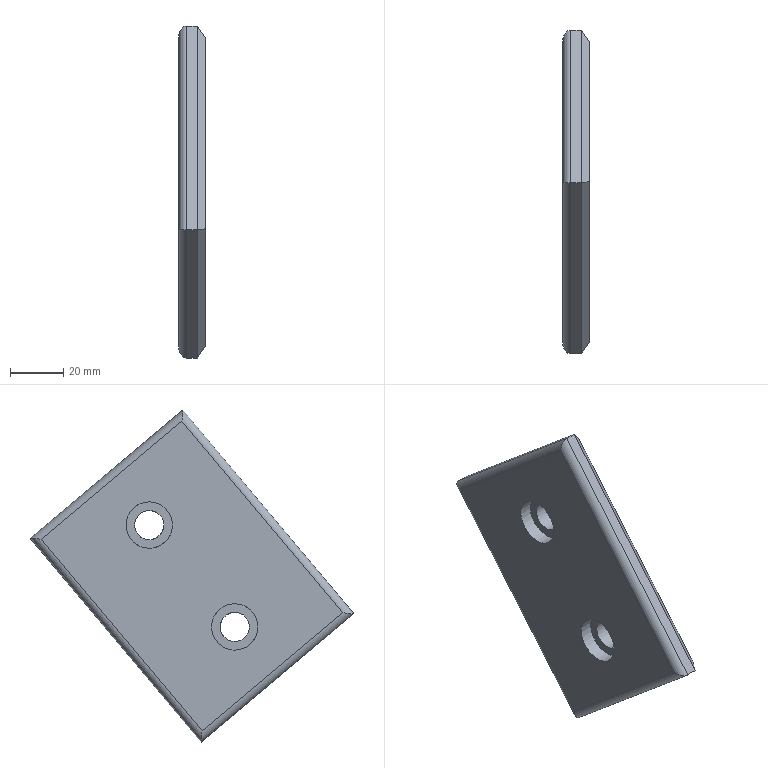Part | NX | features solid 2 | 1 solid | 20 faces | box 10 x 121.732 x 124.814 mm | volume 69440 mm3 | plane 12 | cylinder 8 | commonest cylinder face diameters 6 x4 11 x2 17.5 x2
STEP:
#1=CARTESIAN_POINT('',(-538.,288.281,-130.936));
#2=VERTEX_POINT('',#1);
#3=CARTESIAN_POINT('',(-542.,288.281,-130.936));
#4=VERTEX_POINT('',#3);
#5=CARTESIAN_POINT('',(-535.,288.281,-130.936));
#6=DIRECTION('',(-1.,0.,0.));
#7=VECTOR('',#6,1000.);
#8=LINE('',#5,#7);
#9=EDGE_CURVE('',#2,#4,#8,.T.);
#10=ORIENTED_EDGE('',*,*,#9,.T.);
#11=CARTESIAN_POINT('',(-542.,345.734,-179.146));
#12=VERTEX_POINT('',#11);
#13=CARTESIAN_POINT('',(-542.,288.281,-130.936));
#14=DIRECTION('',(0.,-0.766,0.6428));
#15=VECTOR('',#14,1000.);
#16=LINE('',#13,#15);
#17=EDGE_CURVE('',#12,#4,#16,.T.);
#18=ORIENTED_EDGE('',*,*,#17,.F.);
#19=CARTESIAN_POINT('',(-538.,345.734,-179.146));
#20=VERTEX_POINT('',#19);
#21=CARTESIAN_POINT('',(-535.,345.734,-179.146));
#22=DIRECTION('',(-1.,0.,0.));
#23=VECTOR('',#22,1000.);
#24=LINE('',#21,#23);
#25=EDGE_CURVE('',#20,#12,#24,.T.);
#26=ORIENTED_EDGE('',*,*,#25,.F.);
#27=CARTESIAN_POINT('',(-538.,345.734,-179.146));
#28=DIRECTION('',(0.,0.766,-0.6428));
#29=VECTOR('',#28,1000.);
#30=LINE('',#27,#29);
#31=EDGE_CURVE('',#2,#20,#30,.T.);
#32=ORIENTED_EDGE('',*,*,#31,.F.);
#33=EDGE_LOOP('',(#10,#18,#26,#32));
#34=FACE_BOUND('',#33,.T.);
#35=CARTESIAN_POINT('',(-535.,345.734,-179.146));
#36=DIRECTION('',(0.,0.6428,0.766));
#37=DIRECTION('',(0.,0.766,-0.6428));
#38=AXIS2_PLACEMENT_3D('',#35,#36,#37);
#39=PLANE('',#38);
#40=ADVANCED_FACE('',(#34),#39,.F.);
#41=CARTESIAN_POINT('',(-538.,352.559,-54.332));
#42=VERTEX_POINT('',#41);
#43=CARTESIAN_POINT('',(-542.,352.559,-54.332));
#44=VERTEX_POINT('',#43);
#45=CARTESIAN_POINT('',(-535.,352.559,-54.332));
#46=DIRECTION('',(-1.,0.,0.));
#47=VECTOR('',#46,1000.);
#48=LINE('',#45,#47);
#49=EDGE_CURVE('',#42,#44,#48,.T.);
#50=ORIENTED_EDGE('',*,*,#49,.T.);
#51=CARTESIAN_POINT('',(-542.,352.559,-54.332));
#52=DIRECTION('',(0.,0.6428,0.766));
#53=VECTOR('',#52,1000.);
#54=LINE('',#51,#53);
#55=EDGE_CURVE('',#4,#44,#54,.T.);
#56=ORIENTED_EDGE('',*,*,#55,.F.);
#57=ORIENTED_EDGE('',*,*,#9,.F.);
#58=CARTESIAN_POINT('',(-538.,288.281,-130.936));
#59=DIRECTION('',(0.,-0.6428,-0.766));
#60=VECTOR('',#59,1000.);
#61=LINE('',#58,#60);
#62=EDGE_CURVE('',#42,#2,#61,.T.);
#63=ORIENTED_EDGE('',*,*,#62,.F.);
#64=EDGE_LOOP('',(#50,#56,#57,#63));
#65=FACE_BOUND('',#64,.T.);
#66=CARTESIAN_POINT('',(-535.,288.281,-130.936));
#67=DIRECTION('',(0.,0.766,-0.6428));
#68=DIRECTION('',(1.,0.,0.));
#69=AXIS2_PLACEMENT_3D('',#66,#67,#68);
#70=PLANE('',#69);
#71=ADVANCED_FACE('',(#65),#70,.F.);
#72=CARTESIAN_POINT('',(-538.,410.013,-102.541));
#73=VERTEX_POINT('',#72);
#74=CARTESIAN_POINT('',(-542.,410.013,-102.541));
#75=VERTEX_POINT('',#74);
#76=CARTESIAN_POINT('',(-535.,410.013,-102.541));
#77=DIRECTION('',(-1.,0.,0.));
#78=VECTOR('',#77,1000.);
#79=LINE('',#76,#78);
#80=EDGE_CURVE('',#73,#75,#79,.T.);
#81=ORIENTED_EDGE('',*,*,#80,.T.);
#82=CARTESIAN_POINT('',(-542.,410.013,-102.541));
#83=DIRECTION('',(0.,0.766,-0.6428));
#84=VECTOR('',#83,1000.);
#85=LINE('',#82,#84);
#86=EDGE_CURVE('',#44,#75,#85,.T.);
#87=ORIENTED_EDGE('',*,*,#86,.F.);
#88=ORIENTED_EDGE('',*,*,#49,.F.);
#89=CARTESIAN_POINT('',(-538.,352.559,-54.332));
#90=DIRECTION('',(0.,-0.766,0.6428));
#91=VECTOR('',#90,1000.);
#92=LINE('',#89,#91);
#93=EDGE_CURVE('',#73,#42,#92,.T.);
#94=ORIENTED_EDGE('',*,*,#93,.F.);
#95=EDGE_LOOP('',(#81,#87,#88,#94));
#96=FACE_BOUND('',#95,.T.);
#97=CARTESIAN_POINT('',(-535.,352.559,-54.332));
#98=DIRECTION('',(0.,-0.6428,-0.766));
#99=DIRECTION('',(1.,0.,0.));
#100=AXIS2_PLACEMENT_3D('',#97,#98,#99);
#101=PLANE('',#100);
#102=ADVANCED_FACE('',(#96),#101,.F.);
#103=ORIENTED_EDGE('',*,*,#25,.T.);
#104=CARTESIAN_POINT('',(-542.,345.734,-179.146));
#105=DIRECTION('',(0.,-0.6428,-0.766));
#106=VECTOR('',#105,1000.);
#107=LINE('',#104,#106);
#108=EDGE_CURVE('',#75,#12,#107,.T.);
#109=ORIENTED_EDGE('',*,*,#108,.F.);
#110=ORIENTED_EDGE('',*,*,#80,.F.);
#111=CARTESIAN_POINT('',(-538.,410.013,-102.541));
#112=DIRECTION('',(0.,0.6428,0.766));
#113=VECTOR('',#112,1000.);
#114=LINE('',#111,#113);
#115=EDGE_CURVE('',#20,#73,#114,.T.);
#116=ORIENTED_EDGE('',*,*,#115,.F.);
#117=EDGE_LOOP('',(#103,#109,#110,#116));
#118=FACE_BOUND('',#117,.T.);
#119=CARTESIAN_POINT('',(-535.,410.013,-102.541));
#120=DIRECTION('',(0.,-0.766,0.6428));
#121=DIRECTION('',(0.,0.6428,0.766));
#122=AXIS2_PLACEMENT_3D('',#119,#120,#121);
#123=PLANE('',#122);
#124=ADVANCED_FACE('',(#118),#123,.F.);
#125=CARTESIAN_POINT('',(-535.,292.507,-130.567));
#126=VERTEX_POINT('',#125);
#127=CARTESIAN_POINT('',(-535.,352.929,-58.558));
#128=VERTEX_POINT('',#127);
#129=CARTESIAN_POINT('',(-535.,290.579,-132.865));
#130=DIRECTION('',(0.,0.6428,0.766));
#131=VECTOR('',#130,1000.);
#132=LINE('',#129,#131);
#133=EDGE_CURVE('',#126,#128,#132,.T.);
#134=ORIENTED_EDGE('',*,*,#133,.F.);
#135=CARTESIAN_POINT('',(-535.,345.364,-174.919));
#136=VERTEX_POINT('',#135);
#137=CARTESIAN_POINT('',(-535.,347.662,-176.847));
#138=DIRECTION('',(0.,-0.766,0.6428));
#139=VECTOR('',#138,1000.);
#140=LINE('',#137,#139);
#141=EDGE_CURVE('',#136,#126,#140,.T.);
#142=ORIENTED_EDGE('',*,*,#141,.F.);
#143=CARTESIAN_POINT('',(-535.,405.786,-102.911));
#144=VERTEX_POINT('',#143);
#145=CARTESIAN_POINT('',(-535.,343.436,-177.217));
#146=DIRECTION('',(0.,-0.6428,-0.766));
#147=VECTOR('',#146,1000.);
#148=LINE('',#145,#147);
#149=EDGE_CURVE('',#144,#136,#148,.T.);
#150=ORIENTED_EDGE('',*,*,#149,.F.);
#151=CARTESIAN_POINT('',(-535.,408.084,-104.839));
#152=DIRECTION('',(0.,0.766,-0.6428));
#153=VECTOR('',#152,1000.);
#154=LINE('',#151,#153);
#155=EDGE_CURVE('',#128,#144,#154,.T.);
#156=ORIENTED_EDGE('',*,*,#155,.F.);
#157=EDGE_LOOP('',(#134,#142,#150,#156));
#158=FACE_BOUND('',#157,.T.);
#159=CARTESIAN_POINT('',(-535.,361.681,-101.801));
#160=VERTEX_POINT('',#159);
#161=CARTESIAN_POINT('',(-535.,365.216,-97.588));
#162=DIRECTION('',(1.,0.,0.));
#163=DIRECTION('',(0.,-0.6428,-0.766));
#164=AXIS2_PLACEMENT_3D('',#161,#162,#163);
#165=CIRCLE('',#164,5.5);
#166=EDGE_CURVE('',#160,#160,#165,.T.);
#167=ORIENTED_EDGE('',*,*,#166,.F.);
#168=EDGE_LOOP('',(#167));
#169=FACE_BOUND('',#168,.T.);
#170=CARTESIAN_POINT('',(-535.,329.542,-140.103));
#171=VERTEX_POINT('',#170);
#172=CARTESIAN_POINT('',(-535.,333.077,-135.89));
#173=DIRECTION('',(1.,0.,0.));
#174=DIRECTION('',(0.,-0.6428,-0.766));
#175=AXIS2_PLACEMENT_3D('',#172,#173,#174);
#176=CIRCLE('',#175,5.5);
#177=EDGE_CURVE('',#171,#171,#176,.T.);
#178=ORIENTED_EDGE('',*,*,#177,.F.);
#179=EDGE_LOOP('',(#178));
#180=FACE_BOUND('',#179,.T.);
#181=CARTESIAN_POINT('',(-535.,345.734,-179.146));
#182=DIRECTION('',(-1.,0.,0.));
#183=DIRECTION('',(0.,-0.6428,-0.766));
#184=AXIS2_PLACEMENT_3D('',#181,#182,#183);
#185=PLANE('',#184);
#186=ADVANCED_FACE('',(#158,#169,#180),#185,.F.);
#187=CARTESIAN_POINT('',(-545.,292.507,-130.567));
#188=VERTEX_POINT('',#187);
#189=CARTESIAN_POINT('',(-545.,345.364,-174.919));
#190=VERTEX_POINT('',#189);
#191=CARTESIAN_POINT('',(-545.,347.662,-176.847));
#192=DIRECTION('',(0.,-0.766,0.6428));
#193=VECTOR('',#192,1000.);
#194=LINE('',#191,#193);
#195=EDGE_CURVE('',#188,#190,#194,.F.);
#196=ORIENTED_EDGE('',*,*,#195,.F.);
#197=CARTESIAN_POINT('',(-545.,352.929,-58.558));
#198=VERTEX_POINT('',#197);
#199=CARTESIAN_POINT('',(-545.,290.579,-132.865));
#200=DIRECTION('',(0.,0.6428,0.766));
#201=VECTOR('',#200,1000.);
#202=LINE('',#199,#201);
#203=EDGE_CURVE('',#198,#188,#202,.F.);
#204=ORIENTED_EDGE('',*,*,#203,.F.);
#205=CARTESIAN_POINT('',(-545.,405.786,-102.911));
#206=VERTEX_POINT('',#205);
#207=CARTESIAN_POINT('',(-545.,350.631,-56.63));
#208=DIRECTION('',(0.,0.766,-0.6428));
#209=VECTOR('',#208,1000.);
#210=LINE('',#207,#209);
#211=EDGE_CURVE('',#206,#198,#210,.F.);
#212=ORIENTED_EDGE('',*,*,#211,.F.);
#213=CARTESIAN_POINT('',(-545.,407.714,-100.613));
#214=DIRECTION('',(0.,-0.6428,-0.766));
#215=VECTOR('',#214,1000.);
#216=LINE('',#213,#215);
#217=EDGE_CURVE('',#190,#206,#216,.F.);
#218=ORIENTED_EDGE('',*,*,#217,.F.);
#219=EDGE_LOOP('',(#196,#204,#212,#218));
#220=FACE_BOUND('',#219,.T.);
#221=CARTESIAN_POINT('',(-545.,370.841,-90.885));
#222=VERTEX_POINT('',#221);
#223=CARTESIAN_POINT('',(-545.,365.216,-97.588));
#224=DIRECTION('',(-1.,0.,0.));
#225=DIRECTION('',(0.,0.6428,0.766));
#226=AXIS2_PLACEMENT_3D('',#223,#224,#225);
#227=CIRCLE('',#226,8.75);
#228=EDGE_CURVE('',#222,#222,#227,.T.);
#229=ORIENTED_EDGE('',*,*,#228,.F.);
#230=EDGE_LOOP('',(#229));
#231=FACE_BOUND('',#230,.T.);
#232=CARTESIAN_POINT('',(-545.,338.701,-129.187));
#233=VERTEX_POINT('',#232);
#234=CARTESIAN_POINT('',(-545.,333.077,-135.89));
#235=DIRECTION('',(-1.,0.,0.));
#236=DIRECTION('',(0.,0.6428,0.766));
#237=AXIS2_PLACEMENT_3D('',#234,#235,#236);
#238=CIRCLE('',#237,8.75);
#239=EDGE_CURVE('',#233,#233,#238,.T.);
#240=ORIENTED_EDGE('',*,*,#239,.F.);
#241=EDGE_LOOP('',(#240));
#242=FACE_BOUND('',#241,.T.);
#243=CARTESIAN_POINT('',(-545.,345.734,-179.146));
#244=DIRECTION('',(-1.,0.,0.));
#245=DIRECTION('',(0.,-0.6428,-0.766));
#246=AXIS2_PLACEMENT_3D('',#243,#244,#245);
#247=PLANE('',#246);
#248=ADVANCED_FACE('',(#220,#231,#242),#247,.T.);
#249=CARTESIAN_POINT('',(-540.,327.577,-135.89));
#250=VERTEX_POINT('',#249);
#251=CARTESIAN_POINT('',(-540.,333.077,-135.89));
#252=DIRECTION('',(-1.,0.,0.));
#253=DIRECTION('',(0.,-1.,0.));
#254=AXIS2_PLACEMENT_3D('',#251,#252,#253);
#255=CIRCLE('',#254,5.5);
#256=EDGE_CURVE('',#250,#250,#255,.T.);
#257=ORIENTED_EDGE('',*,*,#256,.T.);
#258=EDGE_LOOP('',(#257));
#259=FACE_BOUND('',#258,.T.);
#260=ORIENTED_EDGE('',*,*,#177,.T.);
#261=EDGE_LOOP('',(#260));
#262=FACE_BOUND('',#261,.T.);
#263=CARTESIAN_POINT('',(-505.,333.077,-135.89));
#264=DIRECTION('',(1.,0.,0.));
#265=DIRECTION('',(0.,0.6428,0.766));
#266=AXIS2_PLACEMENT_3D('',#263,#264,#265);
#267=CYLINDRICAL_SURFACE('',#266,5.5);
#268=ADVANCED_FACE('',(#259,#262),#267,.F.);
#269=ORIENTED_EDGE('',*,*,#256,.F.);
#270=EDGE_LOOP('',(#269));
#271=FACE_BOUND('',#270,.T.);
#272=CARTESIAN_POINT('',(-540.,324.327,-135.89));
#273=VERTEX_POINT('',#272);
#274=CARTESIAN_POINT('',(-540.,333.077,-135.89));
#275=DIRECTION('',(-1.,0.,0.));
#276=DIRECTION('',(0.,-1.,0.));
#277=AXIS2_PLACEMENT_3D('',#274,#275,#276);
#278=CIRCLE('',#277,8.75);
#279=EDGE_CURVE('',#273,#273,#278,.T.);
#280=ORIENTED_EDGE('',*,*,#279,.T.);
#281=EDGE_LOOP('',(#280));
#282=FACE_BOUND('',#281,.T.);
#283=CARTESIAN_POINT('',(-540.,333.077,-135.89));
#284=DIRECTION('',(1.,0.,0.));
#285=DIRECTION('',(0.,0.6428,0.766));
#286=AXIS2_PLACEMENT_3D('',#283,#284,#285);
#287=PLANE('',#286);
#288=ADVANCED_FACE('',(#271,#282),#287,.F.);
#289=ORIENTED_EDGE('',*,*,#279,.F.);
#290=EDGE_LOOP('',(#289));
#291=FACE_BOUND('',#290,.T.);
#292=ORIENTED_EDGE('',*,*,#239,.T.);
#293=EDGE_LOOP('',(#292));
#294=FACE_BOUND('',#293,.T.);
#295=CARTESIAN_POINT('',(-545.,333.077,-135.89));
#296=DIRECTION('',(1.,0.,0.));
#297=DIRECTION('',(0.,0.6428,0.766));
#298=AXIS2_PLACEMENT_3D('',#295,#296,#297);
#299=CYLINDRICAL_SURFACE('',#298,8.75);
#300=ADVANCED_FACE('',(#291,#294),#299,.F.);
#301=CARTESIAN_POINT('',(-540.,359.716,-97.588));
#302=VERTEX_POINT('',#301);
#303=CARTESIAN_POINT('',(-540.,365.216,-97.588));
#304=DIRECTION('',(-1.,0.,0.));
#305=DIRECTION('',(0.,-1.,0.));
#306=AXIS2_PLACEMENT_3D('',#303,#304,#305);
#307=CIRCLE('',#306,5.5);
#308=EDGE_CURVE('',#302,#302,#307,.T.);
#309=ORIENTED_EDGE('',*,*,#308,.T.);
#310=EDGE_LOOP('',(#309));
#311=FACE_BOUND('',#310,.T.);
#312=ORIENTED_EDGE('',*,*,#166,.T.);
#313=EDGE_LOOP('',(#312));
#314=FACE_BOUND('',#313,.T.);
#315=CARTESIAN_POINT('',(-505.,365.216,-97.588));
#316=DIRECTION('',(1.,0.,0.));
#317=DIRECTION('',(0.,0.6428,0.766));
#318=AXIS2_PLACEMENT_3D('',#315,#316,#317);
#319=CYLINDRICAL_SURFACE('',#318,5.5);
#320=ADVANCED_FACE('',(#311,#314),#319,.F.);
#321=ORIENTED_EDGE('',*,*,#308,.F.);
#322=EDGE_LOOP('',(#321));
#323=FACE_BOUND('',#322,.T.);
#324=CARTESIAN_POINT('',(-540.,356.466,-97.588));
#325=VERTEX_POINT('',#324);
#326=CARTESIAN_POINT('',(-540.,365.216,-97.588));
#327=DIRECTION('',(-1.,0.,0.));
#328=DIRECTION('',(0.,-1.,0.));
#329=AXIS2_PLACEMENT_3D('',#326,#327,#328);
#330=CIRCLE('',#329,8.75);
#331=EDGE_CURVE('',#325,#325,#330,.T.);
#332=ORIENTED_EDGE('',*,*,#331,.T.);
#333=EDGE_LOOP('',(#332));
#334=FACE_BOUND('',#333,.T.);
#335=CARTESIAN_POINT('',(-540.,365.216,-97.588));
#336=DIRECTION('',(1.,0.,0.));
#337=DIRECTION('',(0.,0.6428,0.766));
#338=AXIS2_PLACEMENT_3D('',#335,#336,#337);
#339=PLANE('',#338);
#340=ADVANCED_FACE('',(#323,#334),#339,.F.);
#341=ORIENTED_EDGE('',*,*,#331,.F.);
#342=EDGE_LOOP('',(#341));
#343=FACE_BOUND('',#342,.T.);
#344=ORIENTED_EDGE('',*,*,#228,.T.);
#345=EDGE_LOOP('',(#344));
#346=FACE_BOUND('',#345,.T.);
#347=CARTESIAN_POINT('',(-545.,365.216,-97.588));
#348=DIRECTION('',(1.,0.,0.));
#349=DIRECTION('',(0.,0.6428,0.766));
#350=AXIS2_PLACEMENT_3D('',#347,#348,#349);
#351=CYLINDRICAL_SURFACE('',#350,8.75);
#352=ADVANCED_FACE('',(#343,#346),#351,.F.);
#353=CARTESIAN_POINT('',(-542.,292.507,-130.567));
#354=DIRECTION('',(0.,-0.08716,0.9962));
#355=DIRECTION('',(0.,0.9962,0.08716));
#356=AXIS2_PLACEMENT_3D('',#353,#354,#355);
#357=ELLIPSE('',#356,4.243,3.);
#358=EDGE_CURVE('',#188,#4,#357,.T.);
#359=ORIENTED_EDGE('',*,*,#358,.T.);
#360=ORIENTED_EDGE('',*,*,#55,.T.);
#361=CARTESIAN_POINT('',(-542.,352.929,-58.558));
#362=DIRECTION('',(0.,0.9962,0.08716));
#363=DIRECTION('',(0.,0.08716,-0.9962));
#364=AXIS2_PLACEMENT_3D('',#361,#362,#363);
#365=ELLIPSE('',#364,4.243,3.);
#366=EDGE_CURVE('',#44,#198,#365,.F.);
#367=ORIENTED_EDGE('',*,*,#366,.T.);
#368=ORIENTED_EDGE('',*,*,#203,.T.);
#369=EDGE_LOOP('',(#359,#360,#367,#368));
#370=FACE_BOUND('',#369,.T.);
#371=CARTESIAN_POINT('',(-542.,290.579,-132.865));
#372=DIRECTION('',(0.,-0.6428,-0.766));
#373=DIRECTION('',(1.,0.,0.));
#374=AXIS2_PLACEMENT_3D('',#371,#372,#373);
#375=CYLINDRICAL_SURFACE('',#374,3.);
#376=ADVANCED_FACE('',(#370),#375,.T.);
#377=ORIENTED_EDGE('',*,*,#366,.F.);
#378=ORIENTED_EDGE('',*,*,#86,.T.);
#379=CARTESIAN_POINT('',(-542.,405.786,-102.911));
#380=DIRECTION('',(0.,0.08716,-0.9962));
#381=DIRECTION('',(0.,-0.9962,-0.08716));
#382=AXIS2_PLACEMENT_3D('',#379,#380,#381);
#383=ELLIPSE('',#382,4.243,3.);
#384=EDGE_CURVE('',#75,#206,#383,.F.);
#385=ORIENTED_EDGE('',*,*,#384,.T.);
#386=ORIENTED_EDGE('',*,*,#211,.T.);
#387=EDGE_LOOP('',(#377,#378,#385,#386));
#388=FACE_BOUND('',#387,.T.);
#389=CARTESIAN_POINT('',(-542.,350.631,-56.63));
#390=DIRECTION('',(0.,-0.766,0.6428));
#391=DIRECTION('',(-1.,0.,0.));
#392=AXIS2_PLACEMENT_3D('',#389,#390,#391);
#393=CYLINDRICAL_SURFACE('',#392,3.);
#394=ADVANCED_FACE('',(#388),#393,.T.);
#395=ORIENTED_EDGE('',*,*,#358,.F.);
#396=ORIENTED_EDGE('',*,*,#195,.T.);
#397=CARTESIAN_POINT('',(-542.,345.364,-174.919));
#398=DIRECTION('',(0.,-0.9962,-0.08716));
#399=DIRECTION('',(0.,0.08716,-0.9962));
#400=AXIS2_PLACEMENT_3D('',#397,#398,#399);
#401=ELLIPSE('',#400,4.243,3.);
#402=EDGE_CURVE('',#190,#12,#401,.T.);
#403=ORIENTED_EDGE('',*,*,#402,.T.);
#404=ORIENTED_EDGE('',*,*,#17,.T.);
#405=EDGE_LOOP('',(#395,#396,#403,#404));
#406=FACE_BOUND('',#405,.T.);
#407=CARTESIAN_POINT('',(-542.,347.662,-176.847));
#408=DIRECTION('',(0.,0.766,-0.6428));
#409=DIRECTION('',(0.,-0.6428,-0.766));
#410=AXIS2_PLACEMENT_3D('',#407,#408,#409);
#411=CYLINDRICAL_SURFACE('',#410,3.);
#412=ADVANCED_FACE('',(#406),#411,.T.);
#413=ORIENTED_EDGE('',*,*,#384,.F.);
#414=ORIENTED_EDGE('',*,*,#108,.T.);
#415=ORIENTED_EDGE('',*,*,#402,.F.);
#416=ORIENTED_EDGE('',*,*,#217,.T.);
#417=EDGE_LOOP('',(#413,#414,#415,#416));
#418=FACE_BOUND('',#417,.T.);
#419=CARTESIAN_POINT('',(-542.,407.714,-100.613));
#420=DIRECTION('',(0.,0.6428,0.766));
#421=DIRECTION('',(0.,0.766,-0.6428));
#422=AXIS2_PLACEMENT_3D('',#419,#420,#421);
#423=CYLINDRICAL_SURFACE('',#422,3.);
#424=ADVANCED_FACE('',(#418),#423,.T.);
#425=CARTESIAN_POINT('',(-536.,345.487,-176.328));
#426=DIRECTION('',(0.5774,-0.07116,0.8134));
#427=VECTOR('',#426,1000.);
#428=LINE('',#425,#427);
#429=EDGE_CURVE('',#20,#136,#428,.T.);
#430=ORIENTED_EDGE('',*,*,#429,.T.);
#431=ORIENTED_EDGE('',*,*,#141,.T.);
#432=CARTESIAN_POINT('',(-511.,326.319,-127.609));
#433=DIRECTION('',(0.5774,0.8134,0.07116));
#434=VECTOR('',#433,1000.);
#435=LINE('',#432,#434);
#436=EDGE_CURVE('',#126,#2,#435,.F.);
#437=ORIENTED_EDGE('',*,*,#436,.T.);
#438=ORIENTED_EDGE('',*,*,#31,.T.);
#439=EDGE_LOOP('',(#430,#431,#437,#438));
#440=FACE_BOUND('',#439,.T.);
#441=CARTESIAN_POINT('',(-535.,347.662,-176.847));
#442=DIRECTION('',(-0.7071,0.4545,0.5417));
#443=DIRECTION('',(-0.7071,-0.4545,-0.5417));
#444=AXIS2_PLACEMENT_3D('',#441,#442,#443);
#445=PLANE('',#444);
#446=ADVANCED_FACE('',(#440),#445,.F.);
#447=ORIENTED_EDGE('',*,*,#436,.F.);
#448=ORIENTED_EDGE('',*,*,#133,.T.);
#449=CARTESIAN_POINT('',(-502.667,356.914,-104.111));
#450=DIRECTION('',(0.5774,0.07116,-0.8134));
#451=VECTOR('',#450,1000.);
#452=LINE('',#449,#451);
#453=EDGE_CURVE('',#128,#42,#452,.F.);
#454=ORIENTED_EDGE('',*,*,#453,.T.);
#455=ORIENTED_EDGE('',*,*,#62,.T.);
#456=EDGE_LOOP('',(#447,#448,#454,#455));
#457=FACE_BOUND('',#456,.T.);
#458=CARTESIAN_POINT('',(-535.,290.579,-132.865));
#459=DIRECTION('',(-0.7071,0.5417,-0.4545));
#460=DIRECTION('',(0.7071,0.5417,-0.4545));
#461=AXIS2_PLACEMENT_3D('',#458,#459,#460);
#462=PLANE('',#461);
#463=ADVANCED_FACE('',(#457),#462,.F.);
#464=ORIENTED_EDGE('',*,*,#429,.F.);
#465=ORIENTED_EDGE('',*,*,#115,.T.);
#466=CARTESIAN_POINT('',(-502.667,360.234,-106.896));
#467=DIRECTION('',(-0.5774,0.8134,0.07116));
#468=VECTOR('',#467,1000.);
#469=LINE('',#466,#468);
#470=EDGE_CURVE('',#73,#144,#469,.F.);
#471=ORIENTED_EDGE('',*,*,#470,.T.);
#472=ORIENTED_EDGE('',*,*,#149,.T.);
#473=EDGE_LOOP('',(#464,#465,#471,#472));
#474=FACE_BOUND('',#473,.T.);
#475=CARTESIAN_POINT('',(-535.,343.436,-177.217));
#476=DIRECTION('',(-0.7071,-0.5417,0.4545));
#477=DIRECTION('',(-0.7071,0.5417,-0.4545));
#478=AXIS2_PLACEMENT_3D('',#475,#476,#477);
#479=PLANE('',#478);
#480=ADVANCED_FACE('',(#474),#479,.F.);
#481=ORIENTED_EDGE('',*,*,#453,.F.);
#482=ORIENTED_EDGE('',*,*,#155,.T.);
#483=ORIENTED_EDGE('',*,*,#470,.F.);
#484=ORIENTED_EDGE('',*,*,#93,.T.);
#485=EDGE_LOOP('',(#481,#482,#483,#484));
#486=FACE_BOUND('',#485,.T.);
#487=CARTESIAN_POINT('',(-535.,408.084,-104.839));
#488=DIRECTION('',(-0.7071,-0.4545,-0.5417));
#489=DIRECTION('',(0.7071,-0.4545,-0.5417));
#490=AXIS2_PLACEMENT_3D('',#487,#488,#489);
#491=PLANE('',#490);
#492=ADVANCED_FACE('',(#486),#491,.F.);
#493=CLOSED_SHELL('',(#40,#71,#102,#124,#186,#248,#268,#288,#300,#320,#340,#352,#376,#394,#412,#424,#446,#463,#480,#492));
#494=MANIFOLD_SOLID_BREP('',#493);
#495=(LENGTH_UNIT()NAMED_UNIT(*)SI_UNIT(.MILLI.,.METRE.));
#496=UNCERTAINTY_MEASURE_WITH_UNIT(LENGTH_MEASURE(0.00001),#495,'','');
#497=(NAMED_UNIT(*)PLANE_ANGLE_UNIT()SI_UNIT($,.RADIAN.));
#498=(NAMED_UNIT(*)SI_UNIT($,.STERADIAN.)SOLID_ANGLE_UNIT());
#499=(GEOMETRIC_REPRESENTATION_CONTEXT(3)GLOBAL_UNCERTAINTY_ASSIGNED_CONTEXT((#496))GLOBAL_UNIT_ASSIGNED_CONTEXT((#495,#497,#498))REPRESENTATION_CONTEXT('',''));
#500=ADVANCED_BREP_SHAPE_REPRESENTATION('',(#494),#499);